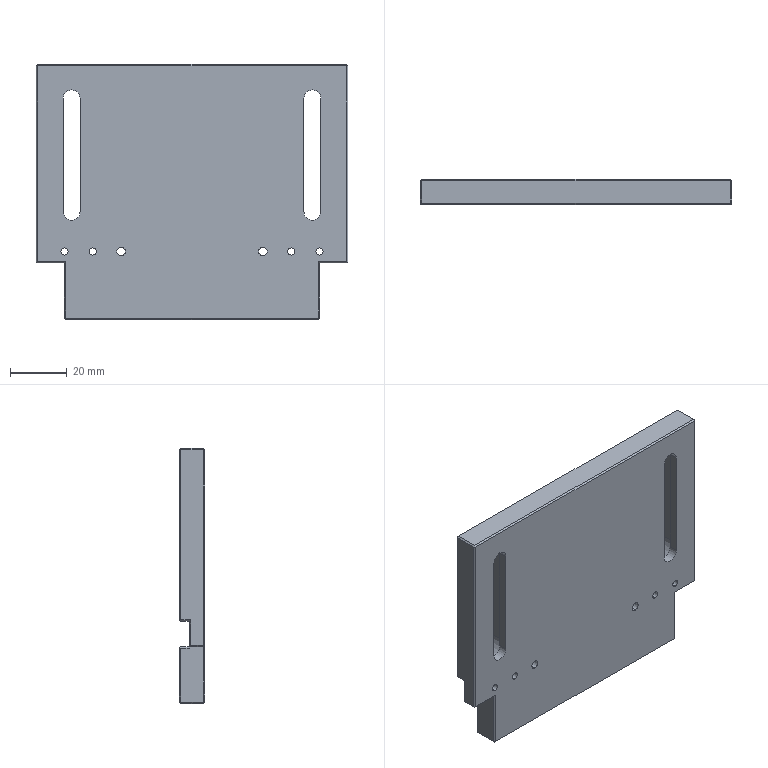Part | SolidWorks | features ICE 6, Chamfer 3, HoleWzd 2, Extrusion 1, MoveFace 1 | 1 solid | 82 faces | box 110 x 9 x 90 mm | volume 72991 mm3 | plane 58 | cylinder 24 | commonest cylinder face diameters 2.5 x8 6 x6 12 x6 3 x4